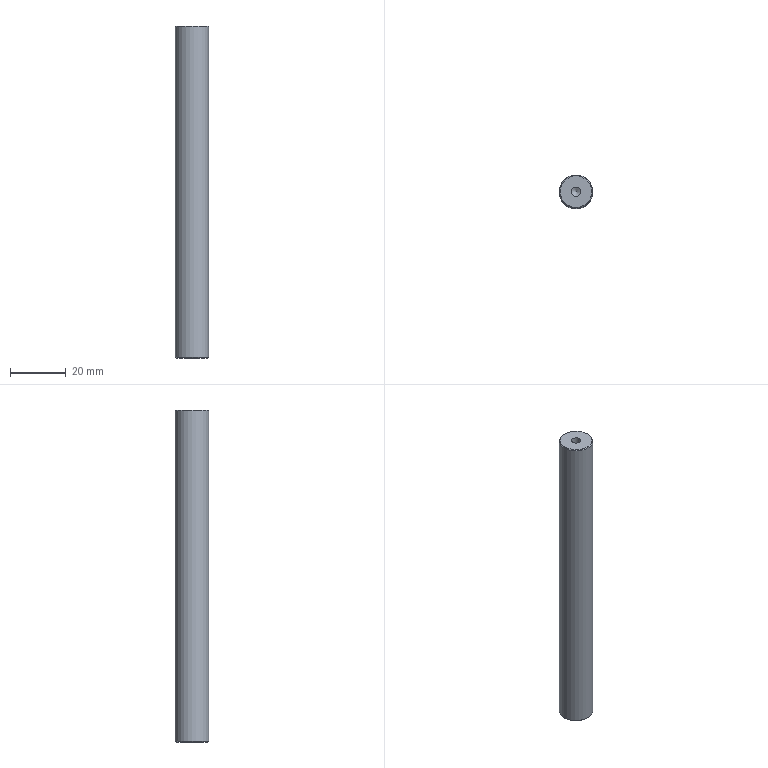Part | NX | 1 solid | 9 faces | box 12 x 12 x 119 mm | volume 13253 mm3 | cone 4 | cylinder 3 | plane 2 | commonest cylinder face diameters 3.3 x2 12 x1
STEP:
#1=CARTESIAN_POINT('',(6.,0.,59.2));
#2=VERTEX_POINT('',#1);
#3=CARTESIAN_POINT('',(0.,0.,59.2));
#4=DIRECTION('',(0.,0.,1.));
#5=DIRECTION('',(1.,0.,0.));
#6=AXIS2_PLACEMENT_3D('',#3,#4,#5);
#7=CIRCLE('',#6,6.);
#8=EDGE_CURVE('',#2,#2,#7,.F.);
#9=ORIENTED_EDGE('',*,*,#8,.T.);
#10=EDGE_LOOP('',(#9));
#11=FACE_BOUND('',#10,.T.);
#12=CARTESIAN_POINT('',(6.,0.,-59.2));
#13=VERTEX_POINT('',#12);
#14=CARTESIAN_POINT('',(0.,0.,-59.2));
#15=DIRECTION('',(0.,0.,1.));
#16=DIRECTION('',(1.,0.,0.));
#17=AXIS2_PLACEMENT_3D('',#14,#15,#16);
#18=CIRCLE('',#17,6.);
#19=EDGE_CURVE('',#13,#13,#18,.T.);
#20=ORIENTED_EDGE('',*,*,#19,.T.);
#21=EDGE_LOOP('',(#20));
#22=FACE_BOUND('',#21,.T.);
#23=CARTESIAN_POINT('',(0.,0.,59.5));
#24=DIRECTION('',(0.,0.,-1.));
#25=DIRECTION('',(-1.,0.,0.));
#26=AXIS2_PLACEMENT_3D('',#23,#24,#25);
#27=CYLINDRICAL_SURFACE('',#26,6.);
#28=ADVANCED_FACE('',(#11,#22),#27,.T.);
#29=CARTESIAN_POINT('',(5.7,0.,59.5));
#30=VERTEX_POINT('',#29);
#31=CARTESIAN_POINT('',(0.,0.,59.5));
#32=DIRECTION('',(0.,0.,1.));
#33=DIRECTION('',(1.,0.,0.));
#34=AXIS2_PLACEMENT_3D('',#31,#32,#33);
#35=CIRCLE('',#34,5.7);
#36=EDGE_CURVE('',#30,#30,#35,.T.);
#37=ORIENTED_EDGE('',*,*,#36,.T.);
#38=EDGE_LOOP('',(#37));
#39=FACE_BOUND('',#38,.T.);
#40=CARTESIAN_POINT('',(1.65,0.,59.5));
#41=VERTEX_POINT('',#40);
#42=CARTESIAN_POINT('',(0.,0.,59.5));
#43=DIRECTION('',(0.,0.,1.));
#44=DIRECTION('',(1.,0.,0.));
#45=AXIS2_PLACEMENT_3D('',#42,#43,#44);
#46=CIRCLE('',#45,1.65);
#47=EDGE_CURVE('',#41,#41,#46,.T.);
#48=ORIENTED_EDGE('',*,*,#47,.F.);
#49=EDGE_LOOP('',(#48));
#50=FACE_BOUND('',#49,.T.);
#51=CARTESIAN_POINT('',(0.,0.,59.5));
#52=DIRECTION('',(0.,0.,1.));
#53=DIRECTION('',(1.,0.,0.));
#54=AXIS2_PLACEMENT_3D('',#51,#52,#53);
#55=PLANE('',#54);
#56=ADVANCED_FACE('',(#39,#50),#55,.T.);
#57=CARTESIAN_POINT('',(5.7,0.,-59.5));
#58=VERTEX_POINT('',#57);
#59=CARTESIAN_POINT('',(0.,0.,-59.5));
#60=DIRECTION('',(0.,0.,1.));
#61=DIRECTION('',(1.,0.,0.));
#62=AXIS2_PLACEMENT_3D('',#59,#60,#61);
#63=CIRCLE('',#62,5.7);
#64=EDGE_CURVE('',#58,#58,#63,.F.);
#65=ORIENTED_EDGE('',*,*,#64,.T.);
#66=EDGE_LOOP('',(#65));
#67=FACE_BOUND('',#66,.T.);
#68=CARTESIAN_POINT('',(-1.65,0.,-59.5));
#69=VERTEX_POINT('',#68);
#70=CARTESIAN_POINT('',(0.,0.,-59.5));
#71=DIRECTION('',(0.,0.,-1.));
#72=DIRECTION('',(-1.,0.,0.));
#73=AXIS2_PLACEMENT_3D('',#70,#71,#72);
#74=CIRCLE('',#73,1.65);
#75=EDGE_CURVE('',#69,#69,#74,.T.);
#76=ORIENTED_EDGE('',*,*,#75,.F.);
#77=EDGE_LOOP('',(#76));
#78=FACE_BOUND('',#77,.T.);
#79=CARTESIAN_POINT('',(0.,0.,-59.5));
#80=DIRECTION('',(0.,0.,1.));
#81=DIRECTION('',(1.,0.,0.));
#82=AXIS2_PLACEMENT_3D('',#79,#80,#81);
#83=PLANE('',#82);
#84=ADVANCED_FACE('',(#67,#78),#83,.F.);
#85=CARTESIAN_POINT('',(0.,0.,-47.009));
#86=VERTEX_POINT('',#85);
#87=VERTEX_LOOP('',#86);
#88=FACE_BOUND('',#87,.T.);
#89=CARTESIAN_POINT('',(-1.65,0.,-48.));
#90=VERTEX_POINT('',#89);
#91=CARTESIAN_POINT('',(0.,0.,-48.));
#92=DIRECTION('',(0.,0.,-1.));
#93=DIRECTION('',(-1.,0.,0.));
#94=AXIS2_PLACEMENT_3D('',#91,#92,#93);
#95=CIRCLE('',#94,1.65);
#96=EDGE_CURVE('',#90,#90,#95,.T.);
#97=ORIENTED_EDGE('',*,*,#96,.T.);
#98=EDGE_LOOP('',(#97));
#99=FACE_BOUND('',#98,.T.);
#100=CARTESIAN_POINT('',(0.,0.,-48.));
#101=DIRECTION('',(0.,0.,-1.));
#102=DIRECTION('',(-1.,0.,0.));
#103=AXIS2_PLACEMENT_3D('',#100,#101,#102);
#104=CONICAL_SURFACE('',#103,1.65,1.03);
#105=ADVANCED_FACE('',(#88,#99),#104,.F.);
#106=ORIENTED_EDGE('',*,*,#96,.F.);
#107=EDGE_LOOP('',(#106));
#108=FACE_BOUND('',#107,.T.);
#109=ORIENTED_EDGE('',*,*,#75,.T.);
#110=EDGE_LOOP('',(#109));
#111=FACE_BOUND('',#110,.T.);
#112=CARTESIAN_POINT('',(0.,0.,-59.5));
#113=DIRECTION('',(0.,0.,-1.));
#114=DIRECTION('',(-1.,0.,0.));
#115=AXIS2_PLACEMENT_3D('',#112,#113,#114);
#116=CYLINDRICAL_SURFACE('',#115,1.65);
#117=ADVANCED_FACE('',(#108,#111),#116,.F.);
#118=CARTESIAN_POINT('',(0.,0.,47.009));
#119=VERTEX_POINT('',#118);
#120=VERTEX_LOOP('',#119);
#121=FACE_BOUND('',#120,.T.);
#122=CARTESIAN_POINT('',(1.65,0.,48.));
#123=VERTEX_POINT('',#122);
#124=CARTESIAN_POINT('',(0.,0.,48.));
#125=DIRECTION('',(0.,0.,1.));
#126=DIRECTION('',(1.,0.,0.));
#127=AXIS2_PLACEMENT_3D('',#124,#125,#126);
#128=CIRCLE('',#127,1.65);
#129=EDGE_CURVE('',#123,#123,#128,.T.);
#130=ORIENTED_EDGE('',*,*,#129,.T.);
#131=EDGE_LOOP('',(#130));
#132=FACE_BOUND('',#131,.T.);
#133=CARTESIAN_POINT('',(0.,0.,48.));
#134=DIRECTION('',(0.,0.,1.));
#135=DIRECTION('',(1.,0.,0.));
#136=AXIS2_PLACEMENT_3D('',#133,#134,#135);
#137=CONICAL_SURFACE('',#136,1.65,1.03);
#138=ADVANCED_FACE('',(#121,#132),#137,.F.);
#139=ORIENTED_EDGE('',*,*,#129,.F.);
#140=EDGE_LOOP('',(#139));
#141=FACE_BOUND('',#140,.T.);
#142=ORIENTED_EDGE('',*,*,#47,.T.);
#143=EDGE_LOOP('',(#142));
#144=FACE_BOUND('',#143,.T.);
#145=CARTESIAN_POINT('',(0.,0.,59.5));
#146=DIRECTION('',(0.,0.,1.));
#147=DIRECTION('',(1.,0.,0.));
#148=AXIS2_PLACEMENT_3D('',#145,#146,#147);
#149=CYLINDRICAL_SURFACE('',#148,1.65);
#150=ADVANCED_FACE('',(#141,#144),#149,.F.);
#151=ORIENTED_EDGE('',*,*,#8,.F.);
#152=EDGE_LOOP('',(#151));
#153=FACE_BOUND('',#152,.T.);
#154=ORIENTED_EDGE('',*,*,#36,.F.);
#155=EDGE_LOOP('',(#154));
#156=FACE_BOUND('',#155,.T.);
#157=CARTESIAN_POINT('',(0.,0.,59.5));
#158=DIRECTION('',(0.,0.,-1.));
#159=DIRECTION('',(-1.,0.,0.));
#160=AXIS2_PLACEMENT_3D('',#157,#158,#159);
#161=CONICAL_SURFACE('',#160,5.7,0.7854);
#162=ADVANCED_FACE('',(#153,#156),#161,.T.);
#163=ORIENTED_EDGE('',*,*,#64,.F.);
#164=EDGE_LOOP('',(#163));
#165=FACE_BOUND('',#164,.T.);
#166=ORIENTED_EDGE('',*,*,#19,.F.);
#167=EDGE_LOOP('',(#166));
#168=FACE_BOUND('',#167,.T.);
#169=CARTESIAN_POINT('',(0.,0.,-59.2));
#170=DIRECTION('',(0.,0.,1.));
#171=DIRECTION('',(1.,0.,0.));
#172=AXIS2_PLACEMENT_3D('',#169,#170,#171);
#173=CONICAL_SURFACE('',#172,6.,0.7854);
#174=ADVANCED_FACE('',(#165,#168),#173,.T.);
#175=CLOSED_SHELL('',(#28,#56,#84,#105,#117,#138,#150,#162,#174));
#176=MANIFOLD_SOLID_BREP('',#175);
#177=(LENGTH_UNIT()NAMED_UNIT(*)SI_UNIT(.MILLI.,.METRE.));
#178=UNCERTAINTY_MEASURE_WITH_UNIT(LENGTH_MEASURE(0.00001),#177,'','');
#179=(NAMED_UNIT(*)PLANE_ANGLE_UNIT()SI_UNIT($,.RADIAN.));
#180=(NAMED_UNIT(*)SI_UNIT($,.STERADIAN.)SOLID_ANGLE_UNIT());
#181=(GEOMETRIC_REPRESENTATION_CONTEXT(3)GLOBAL_UNCERTAINTY_ASSIGNED_CONTEXT((#178))GLOBAL_UNIT_ASSIGNED_CONTEXT((#177,#179,#180))REPRESENTATION_CONTEXT('',''));
#182=ADVANCED_BREP_SHAPE_REPRESENTATION('',(#176),#181);